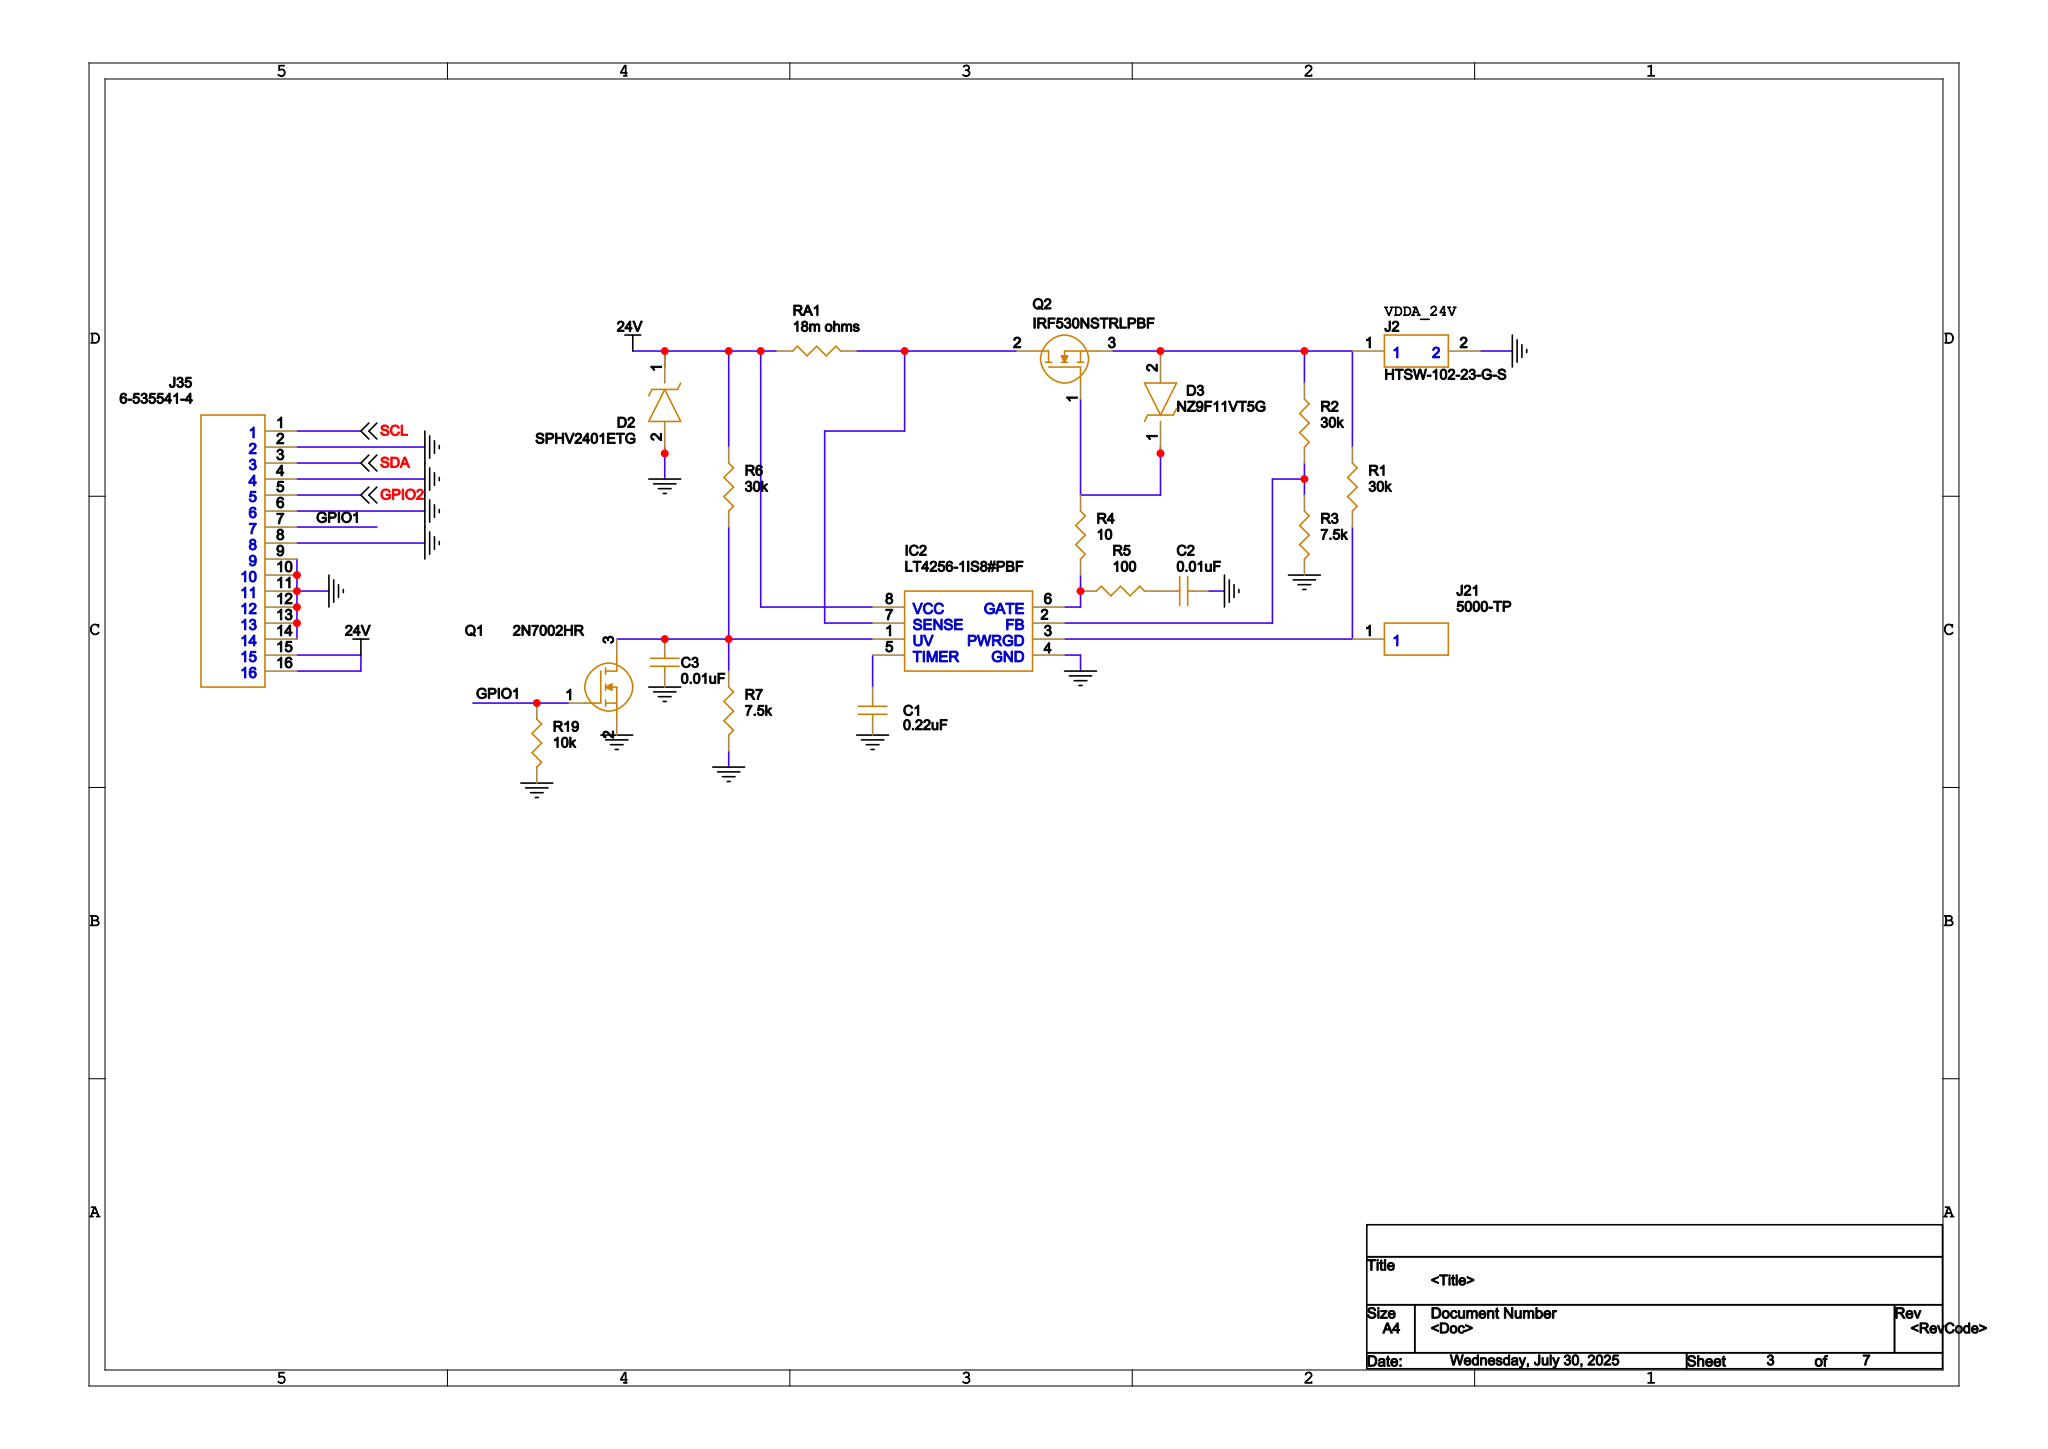Circuit board | Cadence Allegro | 93 parts | 49 nets | one sheet of the schematic
Parts on this sheet (reference | value | footprint):
C1 | 0.22uF | C0402
C2 | 0.01uF | C0402
C3 | 0.01uF | C0402
D2 | SPHV2401ETG | SPHV2401ETG
D3 | NZ9F11VT5G | SOD-923_0P6X0P85_ONS
IC2 | LT4256-1IS8#PBF | SOIC127P599X175-8N
J2 | HTSW-102-23-G-S | HDRV2W64P0X254_1X2_508X248X838P
J21 | 5000-TP | 5000
J35 | 6-535541-4 | DIP-16
Q1 | 2N7002HR | SOT95P230X110-3N
Q2 | IRF530NSTRLPBF | IRF2804STRLPBF
R1 | 30k | R0402
R2 | 30k | R0402
R3 | 7.5k | R0402
R4 | 10 | R0402
R5 | 100 | R0402
R6 | 30k | R0402
R7 | 7.5k | R0402
R19 | 10k | R0402
RA1 | 18m ohms | R0612
Nets of these parts (net: part-pin ...):
24V: D2-1 IC2-8 J35-15 J35-16 R6-1 RA1-1
N00630: IC2-7 Q2-2 RA1-2
GND: C1-2 C2-2 C3-2 D2-2 IC2-4 J2-2 J35-2 J35-4 J35-6 J35-8 J35-9 J35-10 J35-11 J35-12 J35-13 J35-14 Q1-2 R3-2 R7-2 R19-2
SCL: J35-1
SDA: J35-3
GPIO2: J35-5
GPIO1: J35-7 Q1-1 R19-1
N00523: C1-1 IC2-5
N015571: C2-1 R5-2
N00363: C3-1 IC2-1 Q1-3 R6-2 R7-1
N00900: D3-2 J2-1 Q2-3 R1-1 R2-1
N00931: IC2-3 J21-1 R1-2
N01039: IC2-2 R2-2 R3-1
N01530: IC2-6 R4-2 R5-1
N01441: D3-1 Q2-1 R4-1